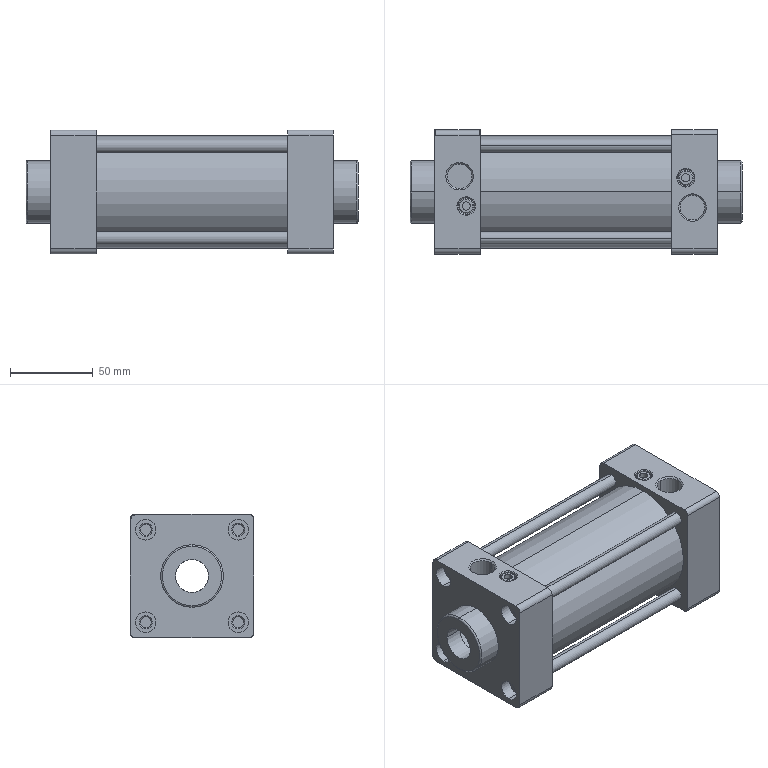Part | SolidWorks | features BaseBody 1 | 1 solid | 160 faces | box 201 x 75 x 75 mm | volume 371064 mm3 | cylinder 80 | plane 46 | cone 30 | torus 4 | commonest cylinder face diameters 6.647 x16 12.5 x16 8 x8 5 x4 6 x4 7 x4